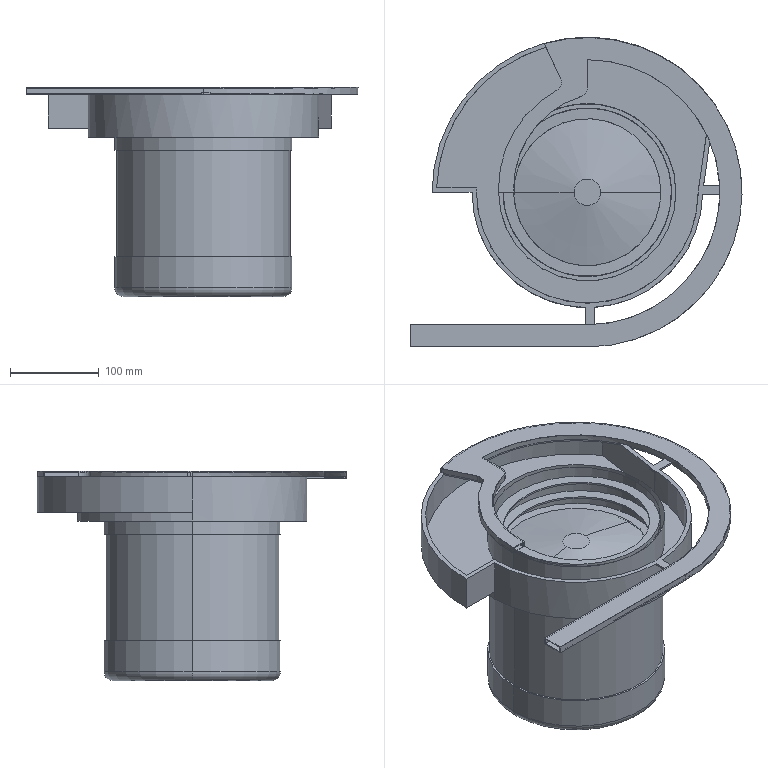Part | SolidWorks | features ICE 7, RevCut 2, Extrusion 1, Fillet 1, Helix 1, Shell 1, Sweep 1 | 4 solids | 108 faces | box 374.5 x 349.5 x 236 mm | volume 6465739 mm3 | plane 64 | cylinder 36 | spline 4 | cone 2 | torus 2 | commonest cylinder face diameters 200 x7 250 x5 190 x3 20 x2 196 x2 216 x2